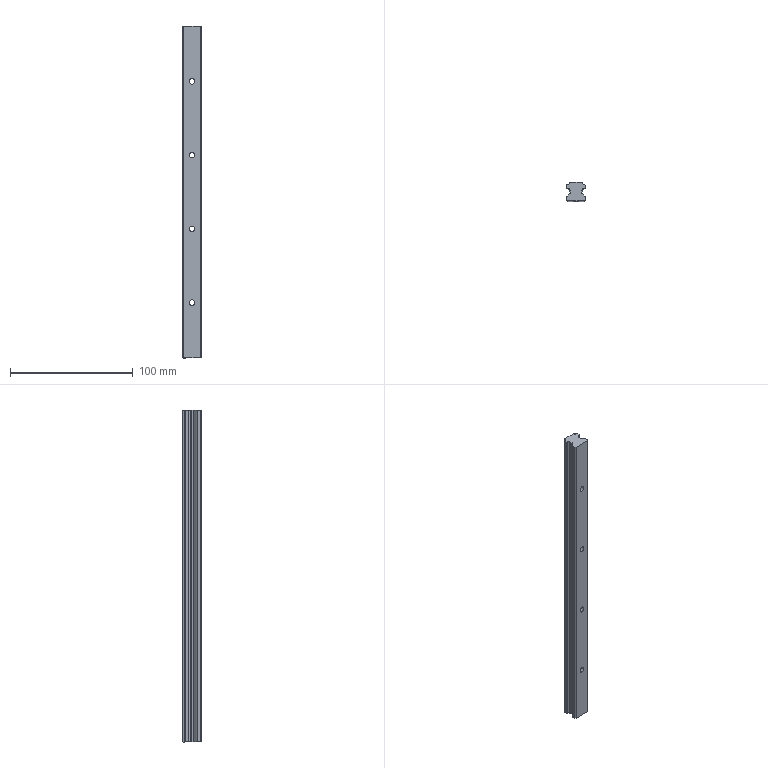Part | SolidWorks | features Draft 2, Fillet 2, ICE 2, Chamfer 1, Extrusion 1, HoleWzd 1 | 1 solid | 56 faces | box 15 x 15 x 270 mm | volume 50125 mm3 | cylinder 30 | plane 26 | commonest cylinder face diameters 0.8 x8 4.5 x8 7.5 x8 3.24 x4 2 x2